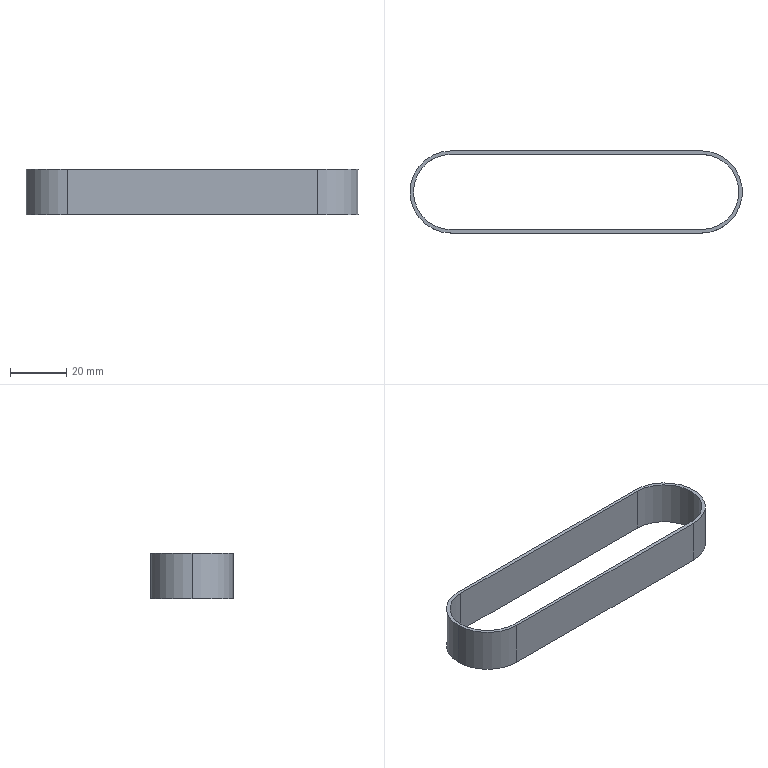Part | STEP file | Timing belt 261-3M-15mm wide_28-28 | 1 solid | 12 faces | box 117.86 x 29.16 x 16 mm | volume 5218 mm3 | cylinder 6 | plane 6 | commonest cylinder face diameters 26.7 x3 29.16 x3
STEP:
#1=CARTESIAN_POINT('',(0.,0.,0.));
#2=DIRECTION('',(0.,0.,1.));
#3=DIRECTION('',(1.,0.,0.));
#4=AXIS2_PLACEMENT_3D('',#1,#2,#3);
#5=CARTESIAN_POINT('',(0.,13.35,8.));
#6=VERTEX_POINT('',#5);
#7=CARTESIAN_POINT('',(0.,13.35,-8.));
#8=VERTEX_POINT('',#7);
#9=CARTESIAN_POINT('',(0.,13.35,8.));
#10=DIRECTION('',(0.,0.,-1.));
#11=VECTOR('',#10,1.);
#12=LINE('',#9,#11);
#13=CARTESIAN_POINT('',(0.,0.,8.));
#14=DIRECTION('',(0.,0.,-1.));
#15=DIRECTION('',(-1.,0.,0.));
#16=AXIS2_PLACEMENT_3D('',#13,#14,#15);
#17=CYLINDRICAL_SURFACE('',#16,13.35);
#18=CARTESIAN_POINT('',(1.571,0.));
#19=DIRECTION('',(0.,1.));
#20=VECTOR('',#19,1.);
#21=LINE('',#18,#20);
#22=(GEOMETRIC_REPRESENTATION_CONTEXT(2)PARAMETRIC_REPRESENTATION_CONTEXT()REPRESENTATION_CONTEXT('',''));
#23=DEFINITIONAL_REPRESENTATION('',(#21),#22);
#24=PCURVE('',#17,#23);
#25=CARTESIAN_POINT('',(0.,13.35,8.));
#26=DIRECTION('',(0.,-1.,0.));
#27=DIRECTION('',(1.,0.,0.));
#28=AXIS2_PLACEMENT_3D('',#25,#26,#27);
#29=PLANE('',#28);
#30=CARTESIAN_POINT('',(0.,0.));
#31=DIRECTION('',(0.,-1.));
#32=VECTOR('',#31,1.);
#33=LINE('',#30,#32);
#34=(GEOMETRIC_REPRESENTATION_CONTEXT(2)PARAMETRIC_REPRESENTATION_CONTEXT()REPRESENTATION_CONTEXT('',''));
#35=DEFINITIONAL_REPRESENTATION('',(#33),#34);
#36=PCURVE('',#29,#35);
#37=SURFACE_CURVE('',#12,(#24,#36),.PCURVE_S1.);
#38=EDGE_CURVE('',#6,#8,#37,.T.);
#39=ORIENTED_EDGE('',*,*,#38,.T.);
#40=CARTESIAN_POINT('',(-13.35,0.,-8.));
#41=VERTEX_POINT('',#40);
#42=CARTESIAN_POINT('',(0.,0.,-8.));
#43=DIRECTION('',(0.,0.,1.));
#44=DIRECTION('',(1.,0.,0.));
#45=AXIS2_PLACEMENT_3D('',#42,#43,#44);
#46=CIRCLE('',#45,13.35);
#47=CARTESIAN_POINT('',(3.142,16.));
#48=DIRECTION('',(-1.,0.));
#49=VECTOR('',#48,1.);
#50=LINE('',#47,#49);
#51=(GEOMETRIC_REPRESENTATION_CONTEXT(2)PARAMETRIC_REPRESENTATION_CONTEXT()REPRESENTATION_CONTEXT('',''));
#52=DEFINITIONAL_REPRESENTATION('',(#50),#51);
#53=PCURVE('',#17,#52);
#54=CARTESIAN_POINT('',(0.,0.,-8.));
#55=DIRECTION('',(0.,0.,1.));
#56=DIRECTION('',(1.,0.,0.));
#57=AXIS2_PLACEMENT_3D('',#54,#55,#56);
#58=PLANE('',#57);
#59=CARTESIAN_POINT('',(0.,0.));
#60=DIRECTION('',(1.,0.));
#61=AXIS2_PLACEMENT_2D('',#59,#60);
#62=CIRCLE('',#61,13.35);
#63=(GEOMETRIC_REPRESENTATION_CONTEXT(2)PARAMETRIC_REPRESENTATION_CONTEXT()REPRESENTATION_CONTEXT('',''));
#64=DEFINITIONAL_REPRESENTATION('',(#62),#63);
#65=PCURVE('',#58,#64);
#66=SURFACE_CURVE('',#46,(#53,#65),.PCURVE_S1.);
#67=EDGE_CURVE('',#8,#41,#66,.T.);
#68=ORIENTED_EDGE('',*,*,#67,.T.);
#69=CARTESIAN_POINT('',(-13.35,0.,8.));
#70=VERTEX_POINT('',#69);
#71=CARTESIAN_POINT('',(-13.35,0.,8.));
#72=DIRECTION('',(0.,0.,-1.));
#73=VECTOR('',#72,1.);
#74=LINE('',#71,#73);
#75=CARTESIAN_POINT('',(0.,0.));
#76=DIRECTION('',(0.,1.));
#77=VECTOR('',#76,1.);
#78=LINE('',#75,#77);
#79=(GEOMETRIC_REPRESENTATION_CONTEXT(2)PARAMETRIC_REPRESENTATION_CONTEXT()REPRESENTATION_CONTEXT('',''));
#80=DEFINITIONAL_REPRESENTATION('',(#78),#79);
#81=PCURVE('',#17,#80);
#82=CARTESIAN_POINT('',(0.,0.,8.));
#83=DIRECTION('',(0.,0.,-1.));
#84=DIRECTION('',(-1.,0.,0.));
#85=AXIS2_PLACEMENT_3D('',#82,#83,#84);
#86=CYLINDRICAL_SURFACE('',#85,13.35);
#87=CARTESIAN_POINT('',(6.283,0.));
#88=DIRECTION('',(0.,1.));
#89=VECTOR('',#88,1.);
#90=LINE('',#87,#89);
#91=(GEOMETRIC_REPRESENTATION_CONTEXT(2)PARAMETRIC_REPRESENTATION_CONTEXT()REPRESENTATION_CONTEXT('',''));
#92=DEFINITIONAL_REPRESENTATION('',(#90),#91);
#93=PCURVE('',#86,#92);
#94=SURFACE_CURVE('',#74,(#81,#93),.PCURVE_S1.);
#95=EDGE_CURVE('',#70,#41,#94,.T.);
#96=ORIENTED_EDGE('',*,*,#95,.F.);
#97=CARTESIAN_POINT('',(0.,0.,8.));
#98=DIRECTION('',(0.,0.,1.));
#99=DIRECTION('',(1.,0.,0.));
#100=AXIS2_PLACEMENT_3D('',#97,#98,#99);
#101=CIRCLE('',#100,13.35);
#102=CARTESIAN_POINT('',(3.142,0.));
#103=DIRECTION('',(-1.,0.));
#104=VECTOR('',#103,1.);
#105=LINE('',#102,#104);
#106=(GEOMETRIC_REPRESENTATION_CONTEXT(2)PARAMETRIC_REPRESENTATION_CONTEXT()REPRESENTATION_CONTEXT('',''));
#107=DEFINITIONAL_REPRESENTATION('',(#105),#106);
#108=PCURVE('',#17,#107);
#109=CARTESIAN_POINT('',(0.,0.,8.));
#110=DIRECTION('',(0.,0.,1.));
#111=DIRECTION('',(1.,0.,0.));
#112=AXIS2_PLACEMENT_3D('',#109,#110,#111);
#113=PLANE('',#112);
#114=CARTESIAN_POINT('',(0.,0.));
#115=DIRECTION('',(1.,0.));
#116=AXIS2_PLACEMENT_2D('',#114,#115);
#117=CIRCLE('',#116,13.35);
#118=(GEOMETRIC_REPRESENTATION_CONTEXT(2)PARAMETRIC_REPRESENTATION_CONTEXT()REPRESENTATION_CONTEXT('',''));
#119=DEFINITIONAL_REPRESENTATION('',(#117),#118);
#120=PCURVE('',#113,#119);
#121=SURFACE_CURVE('',#101,(#108,#120),.PCURVE_S1.);
#122=EDGE_CURVE('',#6,#70,#121,.T.);
#123=ORIENTED_EDGE('',*,*,#122,.F.);
#124=EDGE_LOOP('',(#39,#68,#96,#123));
#125=FACE_BOUND('',#124,.F.);
#126=ADVANCED_FACE('',(#125),#17,.F.);
#127=CARTESIAN_POINT('',(-14.58,0.,8.));
#128=VERTEX_POINT('',#127);
#129=CARTESIAN_POINT('',(0.,-14.58,8.));
#130=VERTEX_POINT('',#129);
#131=CARTESIAN_POINT('',(0.,0.,8.));
#132=DIRECTION('',(0.,0.,1.));
#133=DIRECTION('',(1.,0.,0.));
#134=AXIS2_PLACEMENT_3D('',#131,#132,#133);
#135=CIRCLE('',#134,14.58);
#136=CARTESIAN_POINT('',(0.,0.,8.));
#137=DIRECTION('',(0.,0.,-1.));
#138=DIRECTION('',(-1.,0.,0.));
#139=AXIS2_PLACEMENT_3D('',#136,#137,#138);
#140=CYLINDRICAL_SURFACE('',#139,14.58);
#141=CARTESIAN_POINT('',(9.425,0.));
#142=DIRECTION('',(-1.,0.));
#143=VECTOR('',#142,1.);
#144=LINE('',#141,#143);
#145=(GEOMETRIC_REPRESENTATION_CONTEXT(2)PARAMETRIC_REPRESENTATION_CONTEXT()REPRESENTATION_CONTEXT('',''));
#146=DEFINITIONAL_REPRESENTATION('',(#144),#145);
#147=PCURVE('',#140,#146);
#148=CARTESIAN_POINT('',(0.,0.));
#149=DIRECTION('',(1.,0.));
#150=AXIS2_PLACEMENT_2D('',#148,#149);
#151=CIRCLE('',#150,14.58);
#152=(GEOMETRIC_REPRESENTATION_CONTEXT(2)PARAMETRIC_REPRESENTATION_CONTEXT()REPRESENTATION_CONTEXT('',''));
#153=DEFINITIONAL_REPRESENTATION('',(#151),#152);
#154=PCURVE('',#113,#153);
#155=SURFACE_CURVE('',#135,(#147,#154),.PCURVE_S1.);
#156=EDGE_CURVE('',#128,#130,#155,.T.);
#157=ORIENTED_EDGE('',*,*,#156,.F.);
#158=CARTESIAN_POINT('',(-14.58,0.,-8.));
#159=VERTEX_POINT('',#158);
#160=CARTESIAN_POINT('',(-14.58,0.,8.));
#161=DIRECTION('',(0.,0.,-1.));
#162=VECTOR('',#161,1.);
#163=LINE('',#160,#162);
#164=CARTESIAN_POINT('',(6.283,0.));
#165=DIRECTION('',(0.,1.));
#166=VECTOR('',#165,1.);
#167=LINE('',#164,#166);
#168=(GEOMETRIC_REPRESENTATION_CONTEXT(2)PARAMETRIC_REPRESENTATION_CONTEXT()REPRESENTATION_CONTEXT('',''));
#169=DEFINITIONAL_REPRESENTATION('',(#167),#168);
#170=PCURVE('',#140,#169);
#171=CARTESIAN_POINT('',(0.,0.,8.));
#172=DIRECTION('',(0.,0.,-1.));
#173=DIRECTION('',(-1.,0.,0.));
#174=AXIS2_PLACEMENT_3D('',#171,#172,#173);
#175=CYLINDRICAL_SURFACE('',#174,14.58);
#176=CARTESIAN_POINT('',(0.,0.));
#177=DIRECTION('',(0.,1.));
#178=VECTOR('',#177,1.);
#179=LINE('',#176,#178);
#180=(GEOMETRIC_REPRESENTATION_CONTEXT(2)PARAMETRIC_REPRESENTATION_CONTEXT()REPRESENTATION_CONTEXT('',''));
#181=DEFINITIONAL_REPRESENTATION('',(#179),#180);
#182=PCURVE('',#175,#181);
#183=SURFACE_CURVE('',#163,(#170,#182),.PCURVE_S1.);
#184=EDGE_CURVE('',#128,#159,#183,.T.);
#185=ORIENTED_EDGE('',*,*,#184,.T.);
#186=CARTESIAN_POINT('',(0.,-14.58,-8.));
#187=VERTEX_POINT('',#186);
#188=CARTESIAN_POINT('',(0.,0.,-8.));
#189=DIRECTION('',(0.,0.,1.));
#190=DIRECTION('',(1.,0.,0.));
#191=AXIS2_PLACEMENT_3D('',#188,#189,#190);
#192=CIRCLE('',#191,14.58);
#193=CARTESIAN_POINT('',(9.425,16.));
#194=DIRECTION('',(-1.,0.));
#195=VECTOR('',#194,1.);
#196=LINE('',#193,#195);
#197=(GEOMETRIC_REPRESENTATION_CONTEXT(2)PARAMETRIC_REPRESENTATION_CONTEXT()REPRESENTATION_CONTEXT('',''));
#198=DEFINITIONAL_REPRESENTATION('',(#196),#197);
#199=PCURVE('',#140,#198);
#200=CARTESIAN_POINT('',(0.,0.));
#201=DIRECTION('',(1.,0.));
#202=AXIS2_PLACEMENT_2D('',#200,#201);
#203=CIRCLE('',#202,14.58);
#204=(GEOMETRIC_REPRESENTATION_CONTEXT(2)PARAMETRIC_REPRESENTATION_CONTEXT()REPRESENTATION_CONTEXT('',''));
#205=DEFINITIONAL_REPRESENTATION('',(#203),#204);
#206=PCURVE('',#58,#205);
#207=SURFACE_CURVE('',#192,(#199,#206),.PCURVE_S1.);
#208=EDGE_CURVE('',#159,#187,#207,.T.);
#209=ORIENTED_EDGE('',*,*,#208,.T.);
#210=CARTESIAN_POINT('',(0.,-14.58,8.));
#211=DIRECTION('',(0.,0.,-1.));
#212=VECTOR('',#211,1.);
#213=LINE('',#210,#212);
#214=CARTESIAN_POINT('',(4.712,0.));
#215=DIRECTION('',(0.,1.));
#216=VECTOR('',#215,1.);
#217=LINE('',#214,#216);
#218=(GEOMETRIC_REPRESENTATION_CONTEXT(2)PARAMETRIC_REPRESENTATION_CONTEXT()REPRESENTATION_CONTEXT('',''));
#219=DEFINITIONAL_REPRESENTATION('',(#217),#218);
#220=PCURVE('',#140,#219);
#221=CARTESIAN_POINT('',(0.,-14.58,8.));
#222=DIRECTION('',(0.,1.,0.));
#223=DIRECTION('',(-1.,0.,0.));
#224=AXIS2_PLACEMENT_3D('',#221,#222,#223);
#225=PLANE('',#224);
#226=CARTESIAN_POINT('',(0.,0.));
#227=DIRECTION('',(0.,-1.));
#228=VECTOR('',#227,1.);
#229=LINE('',#226,#228);
#230=(GEOMETRIC_REPRESENTATION_CONTEXT(2)PARAMETRIC_REPRESENTATION_CONTEXT()REPRESENTATION_CONTEXT('',''));
#231=DEFINITIONAL_REPRESENTATION('',(#229),#230);
#232=PCURVE('',#225,#231);
#233=SURFACE_CURVE('',#213,(#220,#232),.PCURVE_S1.);
#234=EDGE_CURVE('',#130,#187,#233,.T.);
#235=ORIENTED_EDGE('',*,*,#234,.F.);
#236=EDGE_LOOP('',(#157,#185,#209,#235));
#237=FACE_BOUND('',#236,.T.);
#238=ADVANCED_FACE('',(#237),#140,.T.);
#239=CARTESIAN_POINT('',(0.,14.58,8.));
#240=VERTEX_POINT('',#239);
#241=CARTESIAN_POINT('',(0.,0.,8.));
#242=DIRECTION('',(0.,0.,1.));
#243=DIRECTION('',(1.,0.,0.));
#244=AXIS2_PLACEMENT_3D('',#241,#242,#243);
#245=CIRCLE('',#244,14.58);
#246=CARTESIAN_POINT('',(0.,0.));
#247=DIRECTION('',(1.,0.));
#248=AXIS2_PLACEMENT_2D('',#246,#247);
#249=CIRCLE('',#248,14.58);
#250=(GEOMETRIC_REPRESENTATION_CONTEXT(2)PARAMETRIC_REPRESENTATION_CONTEXT()REPRESENTATION_CONTEXT('',''));
#251=DEFINITIONAL_REPRESENTATION('',(#249),#250);
#252=PCURVE('',#113,#251);
#253=CARTESIAN_POINT('',(3.142,0.));
#254=DIRECTION('',(-1.,0.));
#255=VECTOR('',#254,1.);
#256=LINE('',#253,#255);
#257=(GEOMETRIC_REPRESENTATION_CONTEXT(2)PARAMETRIC_REPRESENTATION_CONTEXT()REPRESENTATION_CONTEXT('',''));
#258=DEFINITIONAL_REPRESENTATION('',(#256),#257);
#259=PCURVE('',#175,#258);
#260=SURFACE_CURVE('',#245,(#252,#259),.PCURVE_S1.);
#261=EDGE_CURVE('',#240,#128,#260,.T.);
#262=ORIENTED_EDGE('',*,*,#261,.T.);
#263=ORIENTED_EDGE('',*,*,#156,.T.);
#264=CARTESIAN_POINT('',(88.7,-14.58,8.));
#265=VERTEX_POINT('',#264);
#266=CARTESIAN_POINT('',(0.,-14.58,8.));
#267=DIRECTION('',(1.,0.,0.));
#268=VECTOR('',#267,1.);
#269=LINE('',#266,#268);
#270=CARTESIAN_POINT('',(0.,-14.58));
#271=DIRECTION('',(1.,0.));
#272=VECTOR('',#271,1.);
#273=LINE('',#270,#272);
#274=(GEOMETRIC_REPRESENTATION_CONTEXT(2)PARAMETRIC_REPRESENTATION_CONTEXT()REPRESENTATION_CONTEXT('',''));
#275=DEFINITIONAL_REPRESENTATION('',(#273),#274);
#276=PCURVE('',#113,#275);
#277=CARTESIAN_POINT('',(0.,0.));
#278=DIRECTION('',(-1.,0.));
#279=VECTOR('',#278,1.);
#280=LINE('',#277,#279);
#281=(GEOMETRIC_REPRESENTATION_CONTEXT(2)PARAMETRIC_REPRESENTATION_CONTEXT()REPRESENTATION_CONTEXT('',''));
#282=DEFINITIONAL_REPRESENTATION('',(#280),#281);
#283=PCURVE('',#225,#282);
#284=SURFACE_CURVE('',#269,(#276,#283),.PCURVE_S1.);
#285=EDGE_CURVE('',#130,#265,#284,.T.);
#286=ORIENTED_EDGE('',*,*,#285,.T.);
#287=CARTESIAN_POINT('',(88.7,14.58,8.));
#288=VERTEX_POINT('',#287);
#289=CARTESIAN_POINT('',(88.7,0.,8.));
#290=DIRECTION('',(0.,0.,1.));
#291=DIRECTION('',(-1.,0.,0.));
#292=AXIS2_PLACEMENT_3D('',#289,#290,#291);
#293=CIRCLE('',#292,14.58);
#294=CARTESIAN_POINT('',(88.7,0.));
#295=DIRECTION('',(-1.,0.));
#296=AXIS2_PLACEMENT_2D('',#294,#295);
#297=CIRCLE('',#296,14.58);
#298=(GEOMETRIC_REPRESENTATION_CONTEXT(2)PARAMETRIC_REPRESENTATION_CONTEXT()REPRESENTATION_CONTEXT('',''));
#299=DEFINITIONAL_REPRESENTATION('',(#297),#298);
#300=PCURVE('',#113,#299);
#301=CARTESIAN_POINT('',(88.7,0.,8.));
#302=DIRECTION('',(0.,0.,-1.));
#303=DIRECTION('',(-1.,0.,0.));
#304=AXIS2_PLACEMENT_3D('',#301,#302,#303);
#305=CYLINDRICAL_SURFACE('',#304,14.58);
#306=CARTESIAN_POINT('',(6.283,0.));
#307=DIRECTION('',(-1.,0.));
#308=VECTOR('',#307,1.);
#309=LINE('',#306,#308);
#310=(GEOMETRIC_REPRESENTATION_CONTEXT(2)PARAMETRIC_REPRESENTATION_CONTEXT()REPRESENTATION_CONTEXT('',''));
#311=DEFINITIONAL_REPRESENTATION('',(#309),#310);
#312=PCURVE('',#305,#311);
#313=SURFACE_CURVE('',#293,(#300,#312),.PCURVE_S1.);
#314=EDGE_CURVE('',#265,#288,#313,.T.);
#315=ORIENTED_EDGE('',*,*,#314,.T.);
#316=CARTESIAN_POINT('',(0.,14.58,8.));
#317=DIRECTION('',(-1.,0.,0.));
#318=VECTOR('',#317,1.);
#319=LINE('',#316,#318);
#320=CARTESIAN_POINT('',(0.,14.58));
#321=DIRECTION('',(-1.,0.));
#322=VECTOR('',#321,1.);
#323=LINE('',#320,#322);
#324=(GEOMETRIC_REPRESENTATION_CONTEXT(2)PARAMETRIC_REPRESENTATION_CONTEXT()REPRESENTATION_CONTEXT('',''));
#325=DEFINITIONAL_REPRESENTATION('',(#323),#324);
#326=PCURVE('',#113,#325);
#327=CARTESIAN_POINT('',(0.,14.58,8.));
#328=DIRECTION('',(0.,-1.,0.));
#329=DIRECTION('',(1.,0.,0.));
#330=AXIS2_PLACEMENT_3D('',#327,#328,#329);
#331=PLANE('',#330);
#332=CARTESIAN_POINT('',(0.,0.));
#333=DIRECTION('',(-1.,0.));
#334=VECTOR('',#333,1.);
#335=LINE('',#332,#334);
#336=(GEOMETRIC_REPRESENTATION_CONTEXT(2)PARAMETRIC_REPRESENTATION_CONTEXT()REPRESENTATION_CONTEXT('',''));
#337=DEFINITIONAL_REPRESENTATION('',(#335),#336);
#338=PCURVE('',#331,#337);
#339=SURFACE_CURVE('',#319,(#326,#338),.PCURVE_S1.);
#340=EDGE_CURVE('',#288,#240,#339,.T.);
#341=ORIENTED_EDGE('',*,*,#340,.T.);
#342=EDGE_LOOP('',(#262,#263,#286,#315,#341));
#343=FACE_BOUND('',#342,.T.);
#344=CARTESIAN_POINT('',(0.,-13.35,8.));
#345=VERTEX_POINT('',#344);
#346=CARTESIAN_POINT('',(88.7,-13.35,8.));
#347=VERTEX_POINT('',#346);
#348=CARTESIAN_POINT('',(0.,-13.35,8.));
#349=DIRECTION('',(1.,0.,0.));
#350=VECTOR('',#349,1.);
#351=LINE('',#348,#350);
#352=CARTESIAN_POINT('',(0.,-13.35));
#353=DIRECTION('',(1.,0.));
#354=VECTOR('',#353,1.);
#355=LINE('',#352,#354);
#356=(GEOMETRIC_REPRESENTATION_CONTEXT(2)PARAMETRIC_REPRESENTATION_CONTEXT()REPRESENTATION_CONTEXT('',''));
#357=DEFINITIONAL_REPRESENTATION('',(#355),#356);
#358=PCURVE('',#113,#357);
#359=CARTESIAN_POINT('',(0.,-13.35,8.));
#360=DIRECTION('',(0.,1.,0.));
#361=DIRECTION('',(-1.,0.,0.));
#362=AXIS2_PLACEMENT_3D('',#359,#360,#361);
#363=PLANE('',#362);
#364=CARTESIAN_POINT('',(0.,0.));
#365=DIRECTION('',(-1.,0.));
#366=VECTOR('',#365,1.);
#367=LINE('',#364,#366);
#368=(GEOMETRIC_REPRESENTATION_CONTEXT(2)PARAMETRIC_REPRESENTATION_CONTEXT()REPRESENTATION_CONTEXT('',''));
#369=DEFINITIONAL_REPRESENTATION('',(#367),#368);
#370=PCURVE('',#363,#369);
#371=SURFACE_CURVE('',#351,(#358,#370),.PCURVE_S1.);
#372=EDGE_CURVE('',#345,#347,#371,.T.);
#373=ORIENTED_EDGE('',*,*,#372,.F.);
#374=CARTESIAN_POINT('',(0.,0.,8.));
#375=DIRECTION('',(0.,0.,1.));
#376=DIRECTION('',(1.,0.,0.));
#377=AXIS2_PLACEMENT_3D('',#374,#375,#376);
#378=CIRCLE('',#377,13.35);
#379=CARTESIAN_POINT('',(0.,0.));
#380=DIRECTION('',(1.,0.));
#381=AXIS2_PLACEMENT_2D('',#379,#380);
#382=CIRCLE('',#381,13.35);
#383=(GEOMETRIC_REPRESENTATION_CONTEXT(2)PARAMETRIC_REPRESENTATION_CONTEXT()REPRESENTATION_CONTEXT('',''));
#384=DEFINITIONAL_REPRESENTATION('',(#382),#383);
#385=PCURVE('',#113,#384);
#386=CARTESIAN_POINT('',(9.425,0.));
#387=DIRECTION('',(-1.,0.));
#388=VECTOR('',#387,1.);
#389=LINE('',#386,#388);
#390=(GEOMETRIC_REPRESENTATION_CONTEXT(2)PARAMETRIC_REPRESENTATION_CONTEXT()REPRESENTATION_CONTEXT('',''));
#391=DEFINITIONAL_REPRESENTATION('',(#389),#390);
#392=PCURVE('',#86,#391);
#393=SURFACE_CURVE('',#378,(#385,#392),.PCURVE_S1.);
#394=EDGE_CURVE('',#70,#345,#393,.T.);
#395=ORIENTED_EDGE('',*,*,#394,.F.);
#396=ORIENTED_EDGE('',*,*,#122,.F.);
#397=CARTESIAN_POINT('',(88.7,13.35,8.));
#398=VERTEX_POINT('',#397);
#399=CARTESIAN_POINT('',(0.,13.35,8.));
#400=DIRECTION('',(-1.,0.,0.));
#401=VECTOR('',#400,1.);
#402=LINE('',#399,#401);
#403=CARTESIAN_POINT('',(0.,13.35));
#404=DIRECTION('',(-1.,0.));
#405=VECTOR('',#404,1.);
#406=LINE('',#403,#405);
#407=(GEOMETRIC_REPRESENTATION_CONTEXT(2)PARAMETRIC_REPRESENTATION_CONTEXT()REPRESENTATION_CONTEXT('',''));
#408=DEFINITIONAL_REPRESENTATION('',(#406),#407);
#409=PCURVE('',#113,#408);
#410=CARTESIAN_POINT('',(0.,0.));
#411=DIRECTION('',(-1.,0.));
#412=VECTOR('',#411,1.);
#413=LINE('',#410,#412);
#414=(GEOMETRIC_REPRESENTATION_CONTEXT(2)PARAMETRIC_REPRESENTATION_CONTEXT()REPRESENTATION_CONTEXT('',''));
#415=DEFINITIONAL_REPRESENTATION('',(#413),#414);
#416=PCURVE('',#29,#415);
#417=SURFACE_CURVE('',#402,(#409,#416),.PCURVE_S1.);
#418=EDGE_CURVE('',#398,#6,#417,.T.);
#419=ORIENTED_EDGE('',*,*,#418,.F.);
#420=CARTESIAN_POINT('',(88.7,0.,8.));
#421=DIRECTION('',(0.,0.,1.));
#422=DIRECTION('',(-1.,0.,0.));
#423=AXIS2_PLACEMENT_3D('',#420,#421,#422);
#424=CIRCLE('',#423,13.35);
#425=CARTESIAN_POINT('',(88.7,0.));
#426=DIRECTION('',(-1.,0.));
#427=AXIS2_PLACEMENT_2D('',#425,#426);
#428=CIRCLE('',#427,13.35);
#429=(GEOMETRIC_REPRESENTATION_CONTEXT(2)PARAMETRIC_REPRESENTATION_CONTEXT()REPRESENTATION_CONTEXT('',''));
#430=DEFINITIONAL_REPRESENTATION('',(#428),#429);
#431=PCURVE('',#113,#430);
#432=CARTESIAN_POINT('',(88.7,0.,8.));
#433=DIRECTION('',(0.,0.,-1.));
#434=DIRECTION('',(-1.,0.,0.));
#435=AXIS2_PLACEMENT_3D('',#432,#433,#434);
#436=CYLINDRICAL_SURFACE('',#435,13.35);
#437=CARTESIAN_POINT('',(6.283,0.));
#438=DIRECTION('',(-1.,0.));
#439=VECTOR('',#438,1.);
#440=LINE('',#437,#439);
#441=(GEOMETRIC_REPRESENTATION_CONTEXT(2)PARAMETRIC_REPRESENTATION_CONTEXT()REPRESENTATION_CONTEXT('',''));
#442=DEFINITIONAL_REPRESENTATION('',(#440),#441);
#443=PCURVE('',#436,#442);
#444=SURFACE_CURVE('',#424,(#431,#443),.PCURVE_S1.);
#445=EDGE_CURVE('',#347,#398,#444,.T.);
#446=ORIENTED_EDGE('',*,*,#445,.F.);
#447=EDGE_LOOP('',(#373,#395,#396,#419,#446));
#448=FACE_BOUND('',#447,.T.);
#449=ADVANCED_FACE('',(#343,#448),#113,.T.);
#450=CARTESIAN_POINT('',(0.,14.58,-8.));
#451=VERTEX_POINT('',#450);
#452=CARTESIAN_POINT('',(0.,0.,-8.));
#453=DIRECTION('',(0.,0.,1.));
#454=DIRECTION('',(1.,0.,0.));
#455=AXIS2_PLACEMENT_3D('',#452,#453,#454);
#456=CIRCLE('',#455,14.58);
#457=CARTESIAN_POINT('',(0.,0.));
#458=DIRECTION('',(1.,0.));
#459=AXIS2_PLACEMENT_2D('',#457,#458);
#460=CIRCLE('',#459,14.58);
#461=(GEOMETRIC_REPRESENTATION_CONTEXT(2)PARAMETRIC_REPRESENTATION_CONTEXT()REPRESENTATION_CONTEXT('',''));
#462=DEFINITIONAL_REPRESENTATION('',(#460),#461);
#463=PCURVE('',#58,#462);
#464=CARTESIAN_POINT('',(3.142,16.));
#465=DIRECTION('',(-1.,0.));
#466=VECTOR('',#465,1.);
#467=LINE('',#464,#466);
#468=(GEOMETRIC_REPRESENTATION_CONTEXT(2)PARAMETRIC_REPRESENTATION_CONTEXT()REPRESENTATION_CONTEXT('',''));
#469=DEFINITIONAL_REPRESENTATION('',(#467),#468);
#470=PCURVE('',#175,#469);
#471=SURFACE_CURVE('',#456,(#463,#470),.PCURVE_S1.);
#472=EDGE_CURVE('',#451,#159,#471,.T.);
#473=ORIENTED_EDGE('',*,*,#472,.F.);
#474=CARTESIAN_POINT('',(88.7,14.58,-8.));
#475=VERTEX_POINT('',#474);
#476=CARTESIAN_POINT('',(0.,14.58,-8.));
#477=DIRECTION('',(-1.,0.,0.));
#478=VECTOR('',#477,1.);
#479=LINE('',#476,#478);
#480=CARTESIAN_POINT('',(0.,14.58));
#481=DIRECTION('',(-1.,0.));
#482=VECTOR('',#481,1.);
#483=LINE('',#480,#482);
#484=(GEOMETRIC_REPRESENTATION_CONTEXT(2)PARAMETRIC_REPRESENTATION_CONTEXT()REPRESENTATION_CONTEXT('',''));
#485=DEFINITIONAL_REPRESENTATION('',(#483),#484);
#486=PCURVE('',#58,#485);
#487=CARTESIAN_POINT('',(0.,-16.));
#488=DIRECTION('',(-1.,0.));
#489=VECTOR('',#488,1.);
#490=LINE('',#487,#489);
#491=(GEOMETRIC_REPRESENTATION_CONTEXT(2)PARAMETRIC_REPRESENTATION_CONTEXT()REPRESENTATION_CONTEXT('',''));
#492=DEFINITIONAL_REPRESENTATION('',(#490),#491);
#493=PCURVE('',#331,#492);
#494=SURFACE_CURVE('',#479,(#486,#493),.PCURVE_S1.);
#495=EDGE_CURVE('',#475,#451,#494,.T.);
#496=ORIENTED_EDGE('',*,*,#495,.F.);
#497=CARTESIAN_POINT('',(88.7,-14.58,-8.));
#498=VERTEX_POINT('',#497);
#499=CARTESIAN_POINT('',(88.7,0.,-8.));
#500=DIRECTION('',(0.,0.,1.));
#501=DIRECTION('',(-1.,0.,0.));
#502=AXIS2_PLACEMENT_3D('',#499,#500,#501);
#503=CIRCLE('',#502,14.58);
#504=CARTESIAN_POINT('',(88.7,0.));
#505=DIRECTION('',(-1.,0.));
#506=AXIS2_PLACEMENT_2D('',#504,#505);
#507=CIRCLE('',#506,14.58);
#508=(GEOMETRIC_REPRESENTATION_CONTEXT(2)PARAMETRIC_REPRESENTATION_CONTEXT()REPRESENTATION_CONTEXT('',''));
#509=DEFINITIONAL_REPRESENTATION('',(#507),#508);
#510=PCURVE('',#58,#509);
#511=CARTESIAN_POINT('',(6.283,16.));
#512=DIRECTION('',(-1.,0.));
#513=VECTOR('',#512,1.);
#514=LINE('',#511,#513);
#515=(GEOMETRIC_REPRESENTATION_CONTEXT(2)PARAMETRIC_REPRESENTATION_CONTEXT()REPRESENTATION_CONTEXT('',''));
#516=DEFINITIONAL_REPRESENTATION('',(#514),#515);
#517=PCURVE('',#305,#516);
#518=SURFACE_CURVE('',#503,(#510,#517),.PCURVE_S1.);
#519=EDGE_CURVE('',#498,#475,#518,.T.);
#520=ORIENTED_EDGE('',*,*,#519,.F.);
#521=CARTESIAN_POINT('',(0.,-14.58,-8.));
#522=DIRECTION('',(1.,0.,0.));
#523=VECTOR('',#522,1.);
#524=LINE('',#521,#523);
#525=CARTESIAN_POINT('',(0.,-14.58));
#526=DIRECTION('',(1.,0.));
#527=VECTOR('',#526,1.);
#528=LINE('',#525,#527);
#529=(GEOMETRIC_REPRESENTATION_CONTEXT(2)PARAMETRIC_REPRESENTATION_CONTEXT()REPRESENTATION_CONTEXT('',''));
#530=DEFINITIONAL_REPRESENTATION('',(#528),#529);
#531=PCURVE('',#58,#530);
#532=CARTESIAN_POINT('',(0.,-16.));
#533=DIRECTION('',(-1.,0.));
#534=VECTOR('',#533,1.);
#535=LINE('',#532,#534);
#536=(GEOMETRIC_REPRESENTATION_CONTEXT(2)PARAMETRIC_REPRESENTATION_CONTEXT()REPRESENTATION_CONTEXT('',''));
#537=DEFINITIONAL_REPRESENTATION('',(#535),#536);
#538=PCURVE('',#225,#537);
#539=SURFACE_CURVE('',#524,(#531,#538),.PCURVE_S1.);
#540=EDGE_CURVE('',#187,#498,#539,.T.);
#541=ORIENTED_EDGE('',*,*,#540,.F.);
#542=ORIENTED_EDGE('',*,*,#208,.F.);
#543=EDGE_LOOP('',(#473,#496,#520,#541,#542));
#544=FACE_BOUND('',#543,.T.);
#545=ORIENTED_EDGE('',*,*,#67,.T.);
#546=CARTESIAN_POINT('',(0.,-13.35,-8.));
#547=VERTEX_POINT('',#546);
#548=CARTESIAN_POINT('',(0.,0.,-8.));
#549=DIRECTION('',(0.,0.,1.));
#550=DIRECTION('',(1.,0.,0.));
#551=AXIS2_PLACEMENT_3D('',#548,#549,#550);
#552=CIRCLE('',#551,13.35);
#553=CARTESIAN_POINT('',(0.,0.));
#554=DIRECTION('',(1.,0.));
#555=AXIS2_PLACEMENT_2D('',#553,#554);
#556=CIRCLE('',#555,13.35);
#557=(GEOMETRIC_REPRESENTATION_CONTEXT(2)PARAMETRIC_REPRESENTATION_CONTEXT()REPRESENTATION_CONTEXT('',''));
#558=DEFINITIONAL_REPRESENTATION('',(#556),#557);
#559=PCURVE('',#58,#558);
#560=CARTESIAN_POINT('',(9.425,16.));
#561=DIRECTION('',(-1.,0.));
#562=VECTOR('',#561,1.);
#563=LINE('',#560,#562);
#564=(GEOMETRIC_REPRESENTATION_CONTEXT(2)PARAMETRIC_REPRESENTATION_CONTEXT()REPRESENTATION_CONTEXT('',''));
#565=DEFINITIONAL_REPRESENTATION('',(#563),#564);
#566=PCURVE('',#86,#565);
#567=SURFACE_CURVE('',#552,(#559,#566),.PCURVE_S1.);
#568=EDGE_CURVE('',#41,#547,#567,.T.);
#569=ORIENTED_EDGE('',*,*,#568,.T.);
#570=CARTESIAN_POINT('',(88.7,-13.35,-8.));
#571=VERTEX_POINT('',#570);
#572=CARTESIAN_POINT('',(0.,-13.35,-8.));
#573=DIRECTION('',(1.,0.,0.));
#574=VECTOR('',#573,1.);
#575=LINE('',#572,#574);
#576=CARTESIAN_POINT('',(0.,-13.35));
#577=DIRECTION('',(1.,0.));
#578=VECTOR('',#577,1.);
#579=LINE('',#576,#578);
#580=(GEOMETRIC_REPRESENTATION_CONTEXT(2)PARAMETRIC_REPRESENTATION_CONTEXT()REPRESENTATION_CONTEXT('',''));
#581=DEFINITIONAL_REPRESENTATION('',(#579),#580);
#582=PCURVE('',#58,#581);
#583=CARTESIAN_POINT('',(0.,-16.));
#584=DIRECTION('',(-1.,0.));
#585=VECTOR('',#584,1.);
#586=LINE('',#583,#585);
#587=(GEOMETRIC_REPRESENTATION_CONTEXT(2)PARAMETRIC_REPRESENTATION_CONTEXT()REPRESENTATION_CONTEXT('',''));
#588=DEFINITIONAL_REPRESENTATION('',(#586),#587);
#589=PCURVE('',#363,#588);
#590=SURFACE_CURVE('',#575,(#582,#589),.PCURVE_S1.);
#591=EDGE_CURVE('',#547,#571,#590,.T.);
#592=ORIENTED_EDGE('',*,*,#591,.T.);
#593=CARTESIAN_POINT('',(88.7,13.35,-8.));
#594=VERTEX_POINT('',#593);
#595=CARTESIAN_POINT('',(88.7,0.,-8.));
#596=DIRECTION('',(0.,0.,1.));
#597=DIRECTION('',(-1.,0.,0.));
#598=AXIS2_PLACEMENT_3D('',#595,#596,#597);
#599=CIRCLE('',#598,13.35);
#600=CARTESIAN_POINT('',(88.7,0.));
#601=DIRECTION('',(-1.,0.));
#602=AXIS2_PLACEMENT_2D('',#600,#601);
#603=CIRCLE('',#602,13.35);
#604=(GEOMETRIC_REPRESENTATION_CONTEXT(2)PARAMETRIC_REPRESENTATION_CONTEXT()REPRESENTATION_CONTEXT('',''));
#605=DEFINITIONAL_REPRESENTATION('',(#603),#604);
#606=PCURVE('',#58,#605);
#607=CARTESIAN_POINT('',(6.283,16.));
#608=DIRECTION('',(-1.,0.));
#609=VECTOR('',#608,1.);
#610=LINE('',#607,#609);
#611=(GEOMETRIC_REPRESENTATION_CONTEXT(2)PARAMETRIC_REPRESENTATION_CONTEXT()REPRESENTATION_CONTEXT('',''));
#612=DEFINITIONAL_REPRESENTATION('',(#610),#611);
#613=PCURVE('',#436,#612);
#614=SURFACE_CURVE('',#599,(#606,#613),.PCURVE_S1.);
#615=EDGE_CURVE('',#571,#594,#614,.T.);
#616=ORIENTED_EDGE('',*,*,#615,.T.);
#617=CARTESIAN_POINT('',(0.,13.35,-8.));
#618=DIRECTION('',(-1.,0.,0.));
#619=VECTOR('',#618,1.);
#620=LINE('',#617,#619);
#621=CARTESIAN_POINT('',(0.,13.35));
#622=DIRECTION('',(-1.,0.));
#623=VECTOR('',#622,1.);
#624=LINE('',#621,#623);
#625=(GEOMETRIC_REPRESENTATION_CONTEXT(2)PARAMETRIC_REPRESENTATION_CONTEXT()REPRESENTATION_CONTEXT('',''));
#626=DEFINITIONAL_REPRESENTATION('',(#624),#625);
#627=PCURVE('',#58,#626);
#628=CARTESIAN_POINT('',(0.,-16.));
#629=DIRECTION('',(-1.,0.));
#630=VECTOR('',#629,1.);
#631=LINE('',#628,#630);
#632=(GEOMETRIC_REPRESENTATION_CONTEXT(2)PARAMETRIC_REPRESENTATION_CONTEXT()REPRESENTATION_CONTEXT('',''));
#633=DEFINITIONAL_REPRESENTATION('',(#631),#632);
#634=PCURVE('',#29,#633);
#635=SURFACE_CURVE('',#620,(#627,#634),.PCURVE_S1.);
#636=EDGE_CURVE('',#594,#8,#635,.T.);
#637=ORIENTED_EDGE('',*,*,#636,.T.);
#638=EDGE_LOOP('',(#545,#569,#592,#616,#637));
#639=FACE_BOUND('',#638,.T.);
#640=ADVANCED_FACE('',(#544,#639),#58,.F.);
#641=ORIENTED_EDGE('',*,*,#184,.F.);
#642=ORIENTED_EDGE('',*,*,#261,.F.);
#643=CARTESIAN_POINT('',(0.,14.58,8.));
#644=DIRECTION('',(0.,0.,-1.));
#645=VECTOR('',#644,1.);
#646=LINE('',#643,#645);
#647=CARTESIAN_POINT('',(1.571,0.));
#648=DIRECTION('',(0.,1.));
#649=VECTOR('',#648,1.);
#650=LINE('',#647,#649);
#651=(GEOMETRIC_REPRESENTATION_CONTEXT(2)PARAMETRIC_REPRESENTATION_CONTEXT()REPRESENTATION_CONTEXT('',''));
#652=DEFINITIONAL_REPRESENTATION('',(#650),#651);
#653=PCURVE('',#175,#652);
#654=CARTESIAN_POINT('',(0.,0.));
#655=DIRECTION('',(0.,-1.));
#656=VECTOR('',#655,1.);
#657=LINE('',#654,#656);
#658=(GEOMETRIC_REPRESENTATION_CONTEXT(2)PARAMETRIC_REPRESENTATION_CONTEXT()REPRESENTATION_CONTEXT('',''));
#659=DEFINITIONAL_REPRESENTATION('',(#657),#658);
#660=PCURVE('',#331,#659);
#661=SURFACE_CURVE('',#646,(#653,#660),.PCURVE_S1.);
#662=EDGE_CURVE('',#240,#451,#661,.T.);
#663=ORIENTED_EDGE('',*,*,#662,.T.);
#664=ORIENTED_EDGE('',*,*,#472,.T.);
#665=EDGE_LOOP('',(#641,#642,#663,#664));
#666=FACE_BOUND('',#665,.T.);
#667=ADVANCED_FACE('',(#666),#175,.T.);
#668=ORIENTED_EDGE('',*,*,#540,.T.);
#669=CARTESIAN_POINT('',(88.7,-14.58,8.));
#670=DIRECTION('',(0.,0.,-1.));
#671=VECTOR('',#670,1.);
#672=LINE('',#669,#671);
#673=CARTESIAN_POINT('',(-88.7,0.));
#674=DIRECTION('',(0.,-1.));
#675=VECTOR('',#674,1.);
#676=LINE('',#673,#675);
#677=(GEOMETRIC_REPRESENTATION_CONTEXT(2)PARAMETRIC_REPRESENTATION_CONTEXT()REPRESENTATION_CONTEXT('',''));
#678=DEFINITIONAL_REPRESENTATION('',(#676),#677);
#679=PCURVE('',#225,#678);
#680=CARTESIAN_POINT('',(4.712,0.));
#681=DIRECTION('',(0.,1.));
#682=VECTOR('',#681,1.);
#683=LINE('',#680,#682);
#684=(GEOMETRIC_REPRESENTATION_CONTEXT(2)PARAMETRIC_REPRESENTATION_CONTEXT()REPRESENTATION_CONTEXT('',''));
#685=DEFINITIONAL_REPRESENTATION('',(#683),#684);
#686=PCURVE('',#305,#685);
#687=SURFACE_CURVE('',#672,(#679,#686),.PCURVE_S1.);
#688=EDGE_CURVE('',#265,#498,#687,.T.);
#689=ORIENTED_EDGE('',*,*,#688,.F.);
#690=ORIENTED_EDGE('',*,*,#285,.F.);
#691=ORIENTED_EDGE('',*,*,#234,.T.);
#692=EDGE_LOOP('',(#668,#689,#690,#691));
#693=FACE_BOUND('',#692,.T.);
#694=ADVANCED_FACE('',(#693),#225,.F.);
#695=ORIENTED_EDGE('',*,*,#519,.T.);
#696=CARTESIAN_POINT('',(88.7,14.58,8.));
#697=DIRECTION('',(0.,0.,-1.));
#698=VECTOR('',#697,1.);
#699=LINE('',#696,#698);
#700=CARTESIAN_POINT('',(1.571,0.));
#701=DIRECTION('',(0.,1.));
#702=VECTOR('',#701,1.);
#703=LINE('',#700,#702);
#704=(GEOMETRIC_REPRESENTATION_CONTEXT(2)PARAMETRIC_REPRESENTATION_CONTEXT()REPRESENTATION_CONTEXT('',''));
#705=DEFINITIONAL_REPRESENTATION('',(#703),#704);
#706=PCURVE('',#305,#705);
#707=CARTESIAN_POINT('',(88.7,0.));
#708=DIRECTION('',(0.,-1.));
#709=VECTOR('',#708,1.);
#710=LINE('',#707,#709);
#711=(GEOMETRIC_REPRESENTATION_CONTEXT(2)PARAMETRIC_REPRESENTATION_CONTEXT()REPRESENTATION_CONTEXT('',''));
#712=DEFINITIONAL_REPRESENTATION('',(#710),#711);
#713=PCURVE('',#331,#712);
#714=SURFACE_CURVE('',#699,(#706,#713),.PCURVE_S1.);
#715=EDGE_CURVE('',#288,#475,#714,.T.);
#716=ORIENTED_EDGE('',*,*,#715,.F.);
#717=ORIENTED_EDGE('',*,*,#314,.F.);
#718=ORIENTED_EDGE('',*,*,#688,.T.);
#719=EDGE_LOOP('',(#695,#716,#717,#718));
#720=FACE_BOUND('',#719,.T.);
#721=ADVANCED_FACE('',(#720),#305,.T.);
#722=ORIENTED_EDGE('',*,*,#495,.T.);
#723=ORIENTED_EDGE('',*,*,#662,.F.);
#724=ORIENTED_EDGE('',*,*,#340,.F.);
#725=ORIENTED_EDGE('',*,*,#715,.T.);
#726=EDGE_LOOP('',(#722,#723,#724,#725));
#727=FACE_BOUND('',#726,.T.);
#728=ADVANCED_FACE('',(#727),#331,.F.);
#729=ORIENTED_EDGE('',*,*,#568,.T.);
#730=CARTESIAN_POINT('',(0.,-13.35,8.));
#731=DIRECTION('',(0.,0.,-1.));
#732=VECTOR('',#731,1.);
#733=LINE('',#730,#732);
#734=CARTESIAN_POINT('',(4.712,0.));
#735=DIRECTION('',(0.,1.));
#736=VECTOR('',#735,1.);
#737=LINE('',#734,#736);
#738=(GEOMETRIC_REPRESENTATION_CONTEXT(2)PARAMETRIC_REPRESENTATION_CONTEXT()REPRESENTATION_CONTEXT('',''));
#739=DEFINITIONAL_REPRESENTATION('',(#737),#738);
#740=PCURVE('',#86,#739);
#741=CARTESIAN_POINT('',(0.,0.));
#742=DIRECTION('',(0.,-1.));
#743=VECTOR('',#742,1.);
#744=LINE('',#741,#743);
#745=(GEOMETRIC_REPRESENTATION_CONTEXT(2)PARAMETRIC_REPRESENTATION_CONTEXT()REPRESENTATION_CONTEXT('',''));
#746=DEFINITIONAL_REPRESENTATION('',(#744),#745);
#747=PCURVE('',#363,#746);
#748=SURFACE_CURVE('',#733,(#740,#747),.PCURVE_S1.);
#749=EDGE_CURVE('',#345,#547,#748,.T.);
#750=ORIENTED_EDGE('',*,*,#749,.F.);
#751=ORIENTED_EDGE('',*,*,#394,.F.);
#752=ORIENTED_EDGE('',*,*,#95,.T.);
#753=EDGE_LOOP('',(#729,#750,#751,#752));
#754=FACE_BOUND('',#753,.F.);
#755=ADVANCED_FACE('',(#754),#86,.F.);
#756=ORIENTED_EDGE('',*,*,#591,.F.);
#757=ORIENTED_EDGE('',*,*,#749,.F.);
#758=ORIENTED_EDGE('',*,*,#372,.T.);
#759=CARTESIAN_POINT('',(88.7,-13.35,8.));
#760=DIRECTION('',(0.,0.,-1.));
#761=VECTOR('',#760,1.);
#762=LINE('',#759,#761);
#763=CARTESIAN_POINT('',(-88.7,0.));
#764=DIRECTION('',(0.,-1.));
#765=VECTOR('',#764,1.);
#766=LINE('',#763,#765);
#767=(GEOMETRIC_REPRESENTATION_CONTEXT(2)PARAMETRIC_REPRESENTATION_CONTEXT()REPRESENTATION_CONTEXT('',''));
#768=DEFINITIONAL_REPRESENTATION('',(#766),#767);
#769=PCURVE('',#363,#768);
#770=CARTESIAN_POINT('',(4.712,0.));
#771=DIRECTION('',(0.,1.));
#772=VECTOR('',#771,1.);
#773=LINE('',#770,#772);
#774=(GEOMETRIC_REPRESENTATION_CONTEXT(2)PARAMETRIC_REPRESENTATION_CONTEXT()REPRESENTATION_CONTEXT('',''));
#775=DEFINITIONAL_REPRESENTATION('',(#773),#774);
#776=PCURVE('',#436,#775);
#777=SURFACE_CURVE('',#762,(#769,#776),.PCURVE_S1.);
#778=EDGE_CURVE('',#347,#571,#777,.T.);
#779=ORIENTED_EDGE('',*,*,#778,.T.);
#780=EDGE_LOOP('',(#756,#757,#758,#779));
#781=FACE_BOUND('',#780,.T.);
#782=ADVANCED_FACE('',(#781),#363,.T.);
#783=CARTESIAN_POINT('',(88.7,13.35,8.));
#784=DIRECTION('',(0.,0.,-1.));
#785=VECTOR('',#784,1.);
#786=LINE('',#783,#785);
#787=CARTESIAN_POINT('',(1.571,0.));
#788=DIRECTION('',(0.,1.));
#789=VECTOR('',#788,1.);
#790=LINE('',#787,#789);
#791=(GEOMETRIC_REPRESENTATION_CONTEXT(2)PARAMETRIC_REPRESENTATION_CONTEXT()REPRESENTATION_CONTEXT('',''));
#792=DEFINITIONAL_REPRESENTATION('',(#790),#791);
#793=PCURVE('',#436,#792);
#794=CARTESIAN_POINT('',(88.7,0.));
#795=DIRECTION('',(0.,-1.));
#796=VECTOR('',#795,1.);
#797=LINE('',#794,#796);
#798=(GEOMETRIC_REPRESENTATION_CONTEXT(2)PARAMETRIC_REPRESENTATION_CONTEXT()REPRESENTATION_CONTEXT('',''));
#799=DEFINITIONAL_REPRESENTATION('',(#797),#798);
#800=PCURVE('',#29,#799);
#801=SURFACE_CURVE('',#786,(#793,#800),.PCURVE_S1.);
#802=EDGE_CURVE('',#398,#594,#801,.T.);
#803=ORIENTED_EDGE('',*,*,#802,.F.);
#804=ORIENTED_EDGE('',*,*,#445,.F.);
#805=ORIENTED_EDGE('',*,*,#778,.T.);
#806=ORIENTED_EDGE('',*,*,#615,.T.);
#807=EDGE_LOOP('',(#803,#804,#805,#806));
#808=FACE_BOUND('',#807,.F.);
#809=ADVANCED_FACE('',(#808),#436,.F.);
#810=ORIENTED_EDGE('',*,*,#636,.F.);
#811=ORIENTED_EDGE('',*,*,#802,.F.);
#812=ORIENTED_EDGE('',*,*,#418,.T.);
#813=ORIENTED_EDGE('',*,*,#38,.T.);
#814=EDGE_LOOP('',(#810,#811,#812,#813));
#815=FACE_BOUND('',#814,.T.);
#816=ADVANCED_FACE('',(#815),#29,.T.);
#817=CLOSED_SHELL('',(#126,#238,#449,#640,#667,#694,#721,#728,#755,#782,#809,#816));
#818=MANIFOLD_SOLID_BREP('',#817);
#819=(LENGTH_UNIT()NAMED_UNIT(*)SI_UNIT(.MILLI.,.METRE.));
#820=UNCERTAINTY_MEASURE_WITH_UNIT(LENGTH_MEASURE(0.0000001),#819,'','');
#821=(NAMED_UNIT(*)PLANE_ANGLE_UNIT()SI_UNIT($,.RADIAN.));
#822=(NAMED_UNIT(*)SI_UNIT($,.STERADIAN.)SOLID_ANGLE_UNIT());
#823=(GEOMETRIC_REPRESENTATION_CONTEXT(3)GLOBAL_UNCERTAINTY_ASSIGNED_CONTEXT((#820))GLOBAL_UNIT_ASSIGNED_CONTEXT((#819,#821,#822))REPRESENTATION_CONTEXT('',''));
#824=ADVANCED_BREP_SHAPE_REPRESENTATION('',(#4,#818),#823);